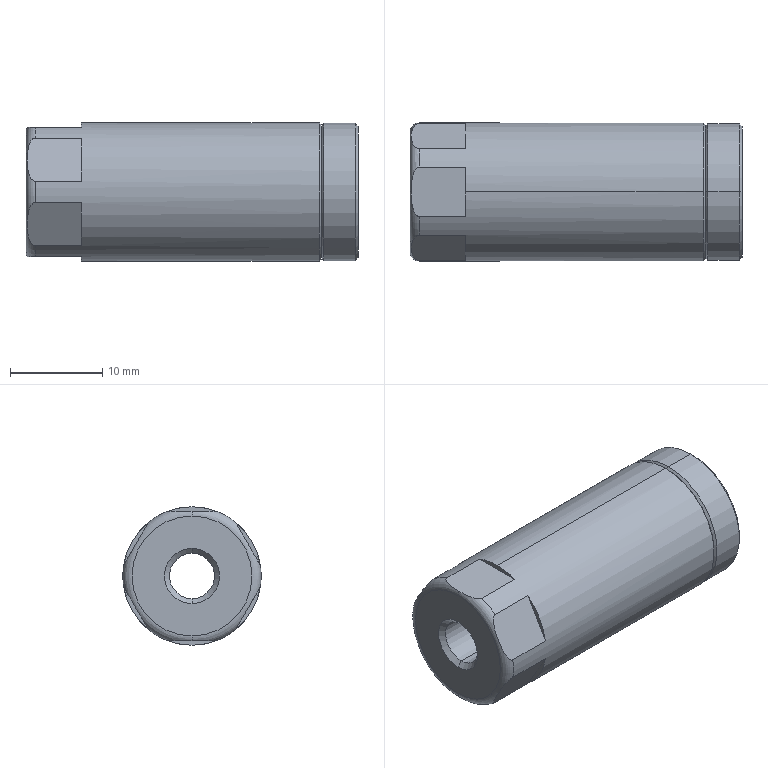Part | STEP file | 1 solid | 35 faces | box 36 x 15 x 15 mm | volume 4516 mm3 | plane 15 | cone 10 | cylinder 8 | torus 2 | commonest cylinder face diameters 4.917 x2 8.5 x2 14.9 x2 15 x2